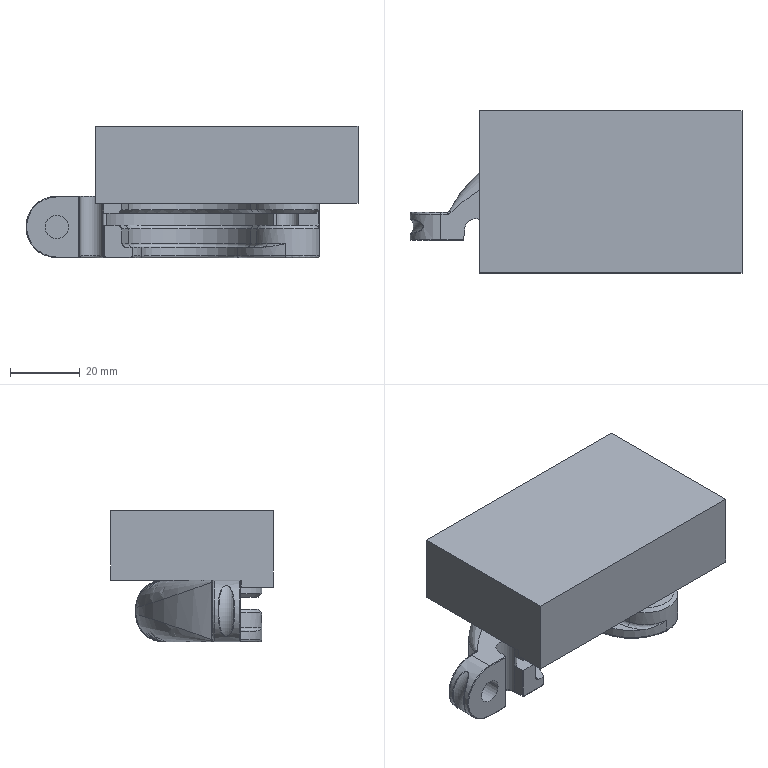Part | 2 solids | 119 faces | box 94.951 x 46.35 x 37.6 mm | volume 89808 mm3 | cylinder 48 | plane 42 | torus 12 | spline 11 | cone 6 | commonest cylinder face diameters 0.4 x8 1 x8 8 x5 18.3 x5 2 x4 6.5 x3